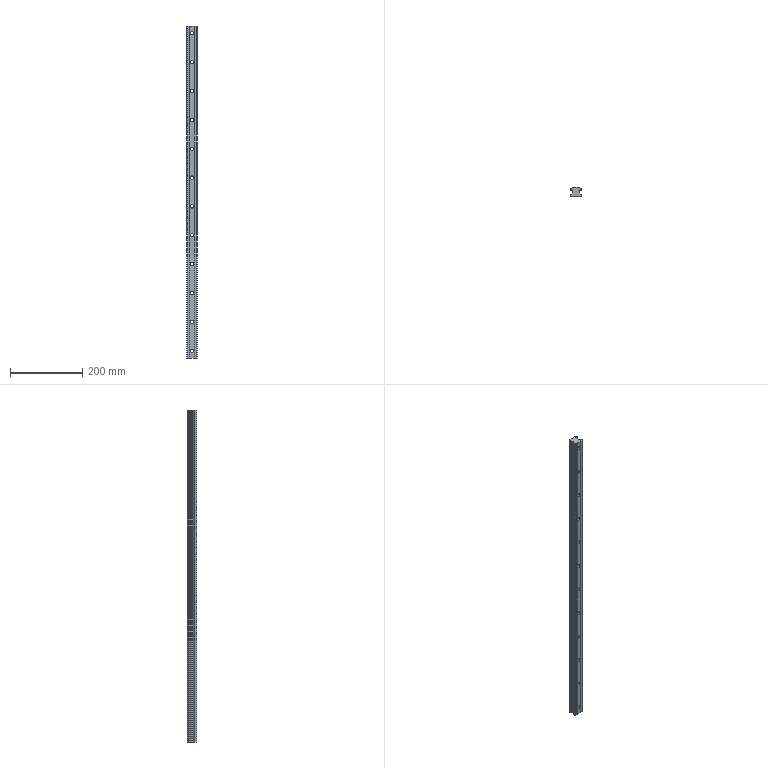Part | SolidWorks | features ICE 2, BaseBody 1, HoleWzd 1 | 1 solid | 112 faces | box 28 x 26 x 920 mm | volume 533776 mm3 | cylinder 70 | plane 42 | commonest cylinder face diameters 9 x24 14 x24 1.2 x12 1.6 x6 5.66 x4